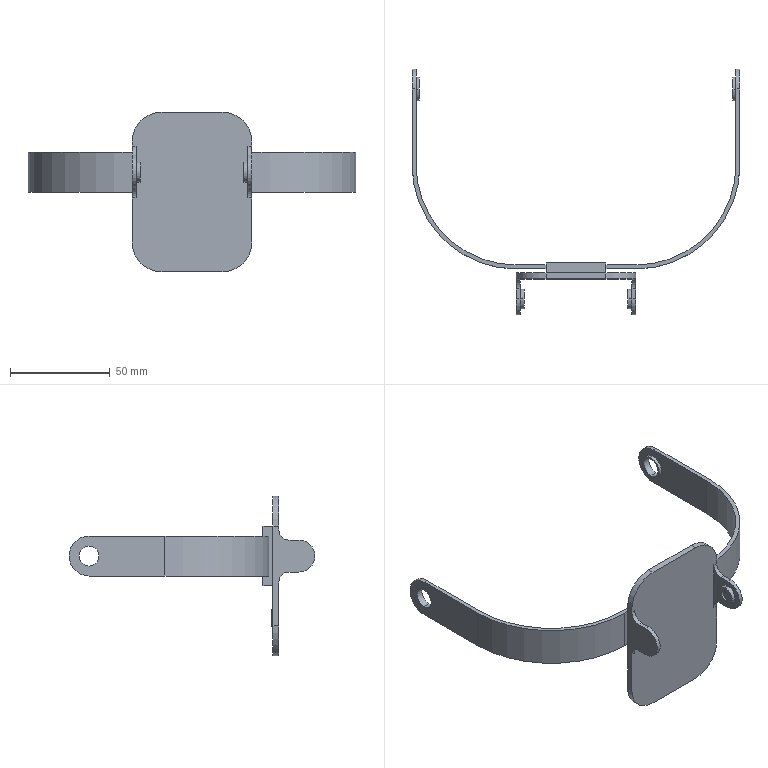Part | SolidWorks | features ICE 13, Extrusion 1, Fillet 1 | 6 solids | 156 faces | box 164 x 123 x 80 mm | volume 30766 mm3 | plane 63 | spline 61 | cylinder 32 | commonest cylinder face diameters 10 x12 5 x4 12 x4 30 x4 16 x2 20 x2